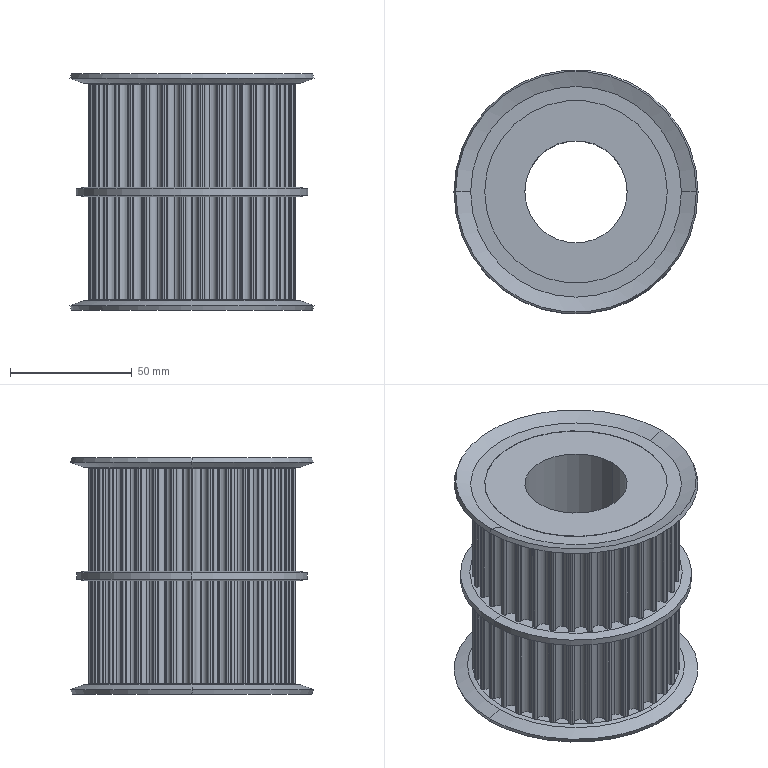Part | SolidWorks | features BaseBody 1 | 1 solid | 712 faces | box 100.208 x 100.208 x 97.168 mm | volume 368257 mm3 | cylinder 414 | plane 278 | cone 16 | spline 4 | commonest cylinder face diameters 1.6 x168 5.14 x168 85.208 x70 75 x4 42 x2 95 x2